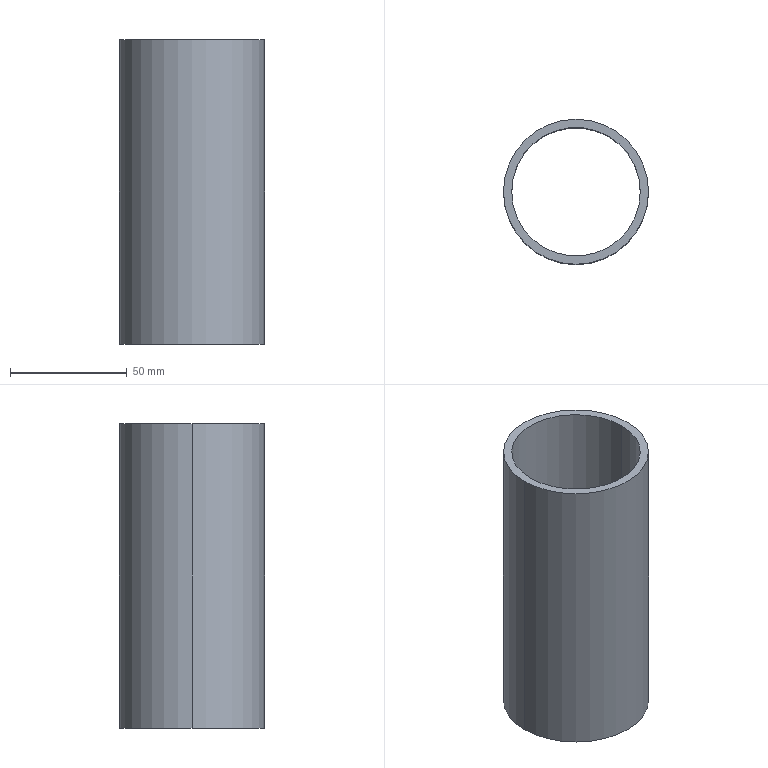Part | SolidWorks | features Extrusion 1 | 1 solid | 6 faces | box 62 x 62 x 130 mm | volume 83621 mm3 | cylinder 4 | plane 2 | commonest cylinder face diameters 55 x2 62 x2
STEP:
#1=CARTESIAN_POINT('',(-27.5,0.,130.));
#2=VERTEX_POINT('',#1);
#3=CARTESIAN_POINT('',(27.5,0.,130.));
#4=VERTEX_POINT('',#3);
#5=CARTESIAN_POINT('',(0.,0.,130.));
#6=DIRECTION('',(0.,0.,1.));
#7=DIRECTION('',(1.,0.,0.));
#8=AXIS2_PLACEMENT_3D('',#5,#6,#7);
#9=CIRCLE('',#8,27.5);
#10=EDGE_CURVE('',#2,#4,#9,.T.);
#11=ORIENTED_EDGE('',*,*,#10,.T.);
#12=CARTESIAN_POINT('',(27.5,0.,0.));
#13=VERTEX_POINT('',#12);
#14=CARTESIAN_POINT('',(27.5,0.,130.));
#15=DIRECTION('',(0.,0.,-1.));
#16=VECTOR('',#15,1000.);
#17=LINE('',#14,#16);
#18=EDGE_CURVE('',#4,#13,#17,.T.);
#19=ORIENTED_EDGE('',*,*,#18,.T.);
#20=CARTESIAN_POINT('',(-27.5,0.,0.));
#21=VERTEX_POINT('',#20);
#22=CARTESIAN_POINT('',(0.,0.,0.));
#23=DIRECTION('',(0.,0.,1.));
#24=DIRECTION('',(1.,0.,0.));
#25=AXIS2_PLACEMENT_3D('',#22,#23,#24);
#26=CIRCLE('',#25,27.5);
#27=EDGE_CURVE('',#21,#13,#26,.T.);
#28=ORIENTED_EDGE('',*,*,#27,.F.);
#29=CARTESIAN_POINT('',(-27.5,0.,130.));
#30=DIRECTION('',(0.,0.,-1.));
#31=VECTOR('',#30,1000.);
#32=LINE('',#29,#31);
#33=EDGE_CURVE('',#2,#21,#32,.T.);
#34=ORIENTED_EDGE('',*,*,#33,.F.);
#35=EDGE_LOOP('',(#11,#19,#28,#34));
#36=FACE_OUTER_BOUND('',#35,.T.);
#37=CARTESIAN_POINT('',(0.,0.,130.));
#38=DIRECTION('',(0.,0.,-1.));
#39=DIRECTION('',(-1.,0.,0.));
#40=AXIS2_PLACEMENT_3D('',#37,#38,#39);
#41=CYLINDRICAL_SURFACE('',#40,27.5);
#42=ADVANCED_FACE('',(#36),#41,.F.);
#43=CARTESIAN_POINT('',(31.,0.,130.));
#44=VERTEX_POINT('',#43);
#45=CARTESIAN_POINT('',(-31.,0.,130.));
#46=VERTEX_POINT('',#45);
#47=CARTESIAN_POINT('',(0.,0.,130.));
#48=DIRECTION('',(0.,0.,1.));
#49=DIRECTION('',(1.,0.,0.));
#50=AXIS2_PLACEMENT_3D('',#47,#48,#49);
#51=CIRCLE('',#50,31.);
#52=EDGE_CURVE('',#44,#46,#51,.T.);
#53=ORIENTED_EDGE('',*,*,#52,.F.);
#54=CARTESIAN_POINT('',(31.,0.,0.));
#55=VERTEX_POINT('',#54);
#56=CARTESIAN_POINT('',(31.,0.,130.));
#57=DIRECTION('',(0.,0.,-1.));
#58=VECTOR('',#57,1000.);
#59=LINE('',#56,#58);
#60=EDGE_CURVE('',#44,#55,#59,.T.);
#61=ORIENTED_EDGE('',*,*,#60,.T.);
#62=CARTESIAN_POINT('',(-31.,0.,0.));
#63=VERTEX_POINT('',#62);
#64=CARTESIAN_POINT('',(0.,0.,0.));
#65=DIRECTION('',(0.,0.,1.));
#66=DIRECTION('',(1.,0.,0.));
#67=AXIS2_PLACEMENT_3D('',#64,#65,#66);
#68=CIRCLE('',#67,31.);
#69=EDGE_CURVE('',#55,#63,#68,.T.);
#70=ORIENTED_EDGE('',*,*,#69,.T.);
#71=CARTESIAN_POINT('',(-31.,0.,130.));
#72=DIRECTION('',(0.,0.,-1.));
#73=VECTOR('',#72,1000.);
#74=LINE('',#71,#73);
#75=EDGE_CURVE('',#46,#63,#74,.T.);
#76=ORIENTED_EDGE('',*,*,#75,.F.);
#77=EDGE_LOOP('',(#53,#61,#70,#76));
#78=FACE_OUTER_BOUND('',#77,.T.);
#79=CARTESIAN_POINT('',(0.,0.,130.));
#80=DIRECTION('',(0.,0.,-1.));
#81=DIRECTION('',(-1.,0.,0.));
#82=AXIS2_PLACEMENT_3D('',#79,#80,#81);
#83=CYLINDRICAL_SURFACE('',#82,31.);
#84=ADVANCED_FACE('',(#78),#83,.T.);
#85=CARTESIAN_POINT('',(0.,0.,130.));
#86=DIRECTION('',(0.,0.,1.));
#87=DIRECTION('',(1.,0.,0.));
#88=AXIS2_PLACEMENT_3D('',#85,#86,#87);
#89=CIRCLE('',#88,31.);
#90=EDGE_CURVE('',#46,#44,#89,.T.);
#91=ORIENTED_EDGE('',*,*,#90,.T.);
#92=ORIENTED_EDGE('',*,*,#52,.T.);
#93=EDGE_LOOP('',(#91,#92));
#94=FACE_OUTER_BOUND('',#93,.T.);
#95=ORIENTED_EDGE('',*,*,#10,.F.);
#96=CARTESIAN_POINT('',(0.,0.,130.));
#97=DIRECTION('',(0.,0.,1.));
#98=DIRECTION('',(1.,0.,0.));
#99=AXIS2_PLACEMENT_3D('',#96,#97,#98);
#100=CIRCLE('',#99,27.5);
#101=EDGE_CURVE('',#4,#2,#100,.T.);
#102=ORIENTED_EDGE('',*,*,#101,.F.);
#103=EDGE_LOOP('',(#95,#102));
#104=FACE_BOUND('',#103,.T.);
#105=CARTESIAN_POINT('',(0.,0.,130.));
#106=DIRECTION('',(0.,0.,1.));
#107=DIRECTION('',(1.,0.,0.));
#108=AXIS2_PLACEMENT_3D('',#105,#106,#107);
#109=PLANE('',#108);
#110=ADVANCED_FACE('',(#94,#104),#109,.T.);
#111=CARTESIAN_POINT('',(0.,0.,0.));
#112=DIRECTION('',(0.,0.,1.));
#113=DIRECTION('',(1.,0.,0.));
#114=AXIS2_PLACEMENT_3D('',#111,#112,#113);
#115=CIRCLE('',#114,31.);
#116=EDGE_CURVE('',#63,#55,#115,.T.);
#117=ORIENTED_EDGE('',*,*,#116,.F.);
#118=ORIENTED_EDGE('',*,*,#69,.F.);
#119=EDGE_LOOP('',(#117,#118));
#120=FACE_OUTER_BOUND('',#119,.T.);
#121=ORIENTED_EDGE('',*,*,#27,.T.);
#122=CARTESIAN_POINT('',(0.,0.,0.));
#123=DIRECTION('',(0.,0.,1.));
#124=DIRECTION('',(1.,0.,0.));
#125=AXIS2_PLACEMENT_3D('',#122,#123,#124);
#126=CIRCLE('',#125,27.5);
#127=EDGE_CURVE('',#13,#21,#126,.T.);
#128=ORIENTED_EDGE('',*,*,#127,.T.);
#129=EDGE_LOOP('',(#121,#128));
#130=FACE_BOUND('',#129,.T.);
#131=CARTESIAN_POINT('',(0.,0.,0.));
#132=DIRECTION('',(0.,0.,1.));
#133=DIRECTION('',(1.,0.,0.));
#134=AXIS2_PLACEMENT_3D('',#131,#132,#133);
#135=PLANE('',#134);
#136=ADVANCED_FACE('',(#120,#130),#135,.F.);
#137=ORIENTED_EDGE('',*,*,#60,.F.);
#138=ORIENTED_EDGE('',*,*,#90,.F.);
#139=ORIENTED_EDGE('',*,*,#75,.T.);
#140=ORIENTED_EDGE('',*,*,#116,.T.);
#141=EDGE_LOOP('',(#137,#138,#139,#140));
#142=FACE_OUTER_BOUND('',#141,.T.);
#143=CARTESIAN_POINT('',(0.,0.,130.));
#144=DIRECTION('',(0.,0.,-1.));
#145=DIRECTION('',(-1.,0.,0.));
#146=AXIS2_PLACEMENT_3D('',#143,#144,#145);
#147=CYLINDRICAL_SURFACE('',#146,31.);
#148=ADVANCED_FACE('',(#142),#147,.T.);
#149=ORIENTED_EDGE('',*,*,#18,.F.);
#150=ORIENTED_EDGE('',*,*,#101,.T.);
#151=ORIENTED_EDGE('',*,*,#33,.T.);
#152=ORIENTED_EDGE('',*,*,#127,.F.);
#153=EDGE_LOOP('',(#149,#150,#151,#152));
#154=FACE_OUTER_BOUND('',#153,.T.);
#155=CARTESIAN_POINT('',(0.,0.,130.));
#156=DIRECTION('',(0.,0.,-1.));
#157=DIRECTION('',(-1.,0.,0.));
#158=AXIS2_PLACEMENT_3D('',#155,#156,#157);
#159=CYLINDRICAL_SURFACE('',#158,27.5);
#160=ADVANCED_FACE('',(#154),#159,.F.);
#161=CLOSED_SHELL('',(#42,#84,#110,#136,#148,#160));
#162=MANIFOLD_SOLID_BREP('',#161);
#163=CARTESIAN_POINT('',(0.,0.,0.));
#164=DIRECTION('',(0.,0.,1.));
#165=DIRECTION('',(1.,0.,0.));
#166=AXIS2_PLACEMENT_3D('',#163,#164,#165);
#167=(LENGTH_UNIT()NAMED_UNIT(*)SI_UNIT(.MILLI.,.METRE.));
#168=UNCERTAINTY_MEASURE_WITH_UNIT(LENGTH_MEASURE(0.00001),#167,'','');
#169=(NAMED_UNIT(*)PLANE_ANGLE_UNIT()SI_UNIT($,.RADIAN.));
#170=(NAMED_UNIT(*)SI_UNIT($,.STERADIAN.)SOLID_ANGLE_UNIT());
#171=(GEOMETRIC_REPRESENTATION_CONTEXT(3)GLOBAL_UNCERTAINTY_ASSIGNED_CONTEXT((#168))GLOBAL_UNIT_ASSIGNED_CONTEXT((#167,#169,#170))REPRESENTATION_CONTEXT('',''));
#172=ADVANCED_BREP_SHAPE_REPRESENTATION('',(#162,#166),#171);